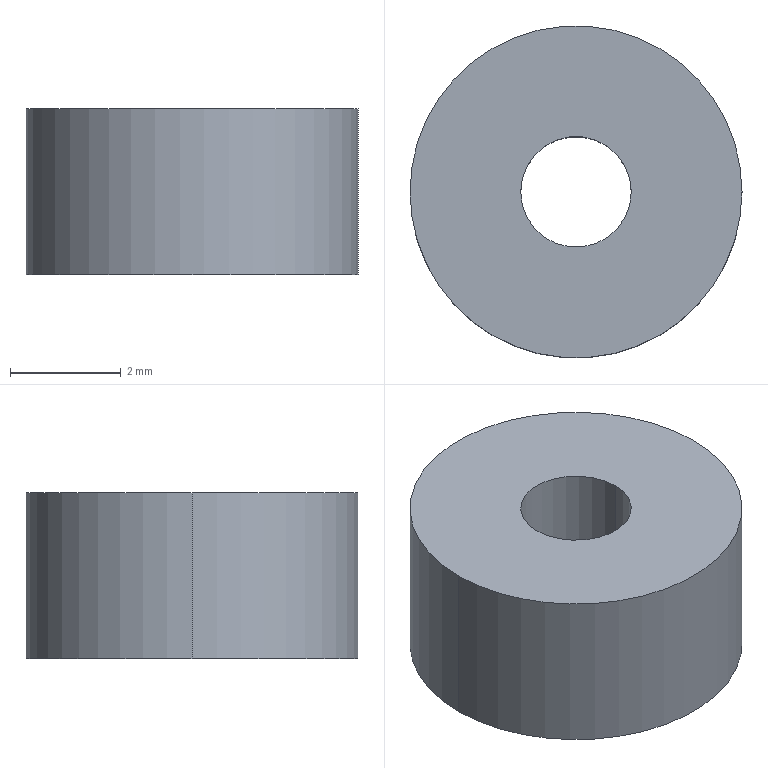Part | STEP file | 1 solid | 6 faces | box 6 x 6 x 3 mm | volume 75.398 mm3 | cylinder 4 | plane 2 | commonest cylinder face diameters 2 x2 6 x2
STEP:
#1=CARTESIAN_POINT('',(0.,0.,0.));
#2=DIRECTION('',(0.,0.,1.));
#3=DIRECTION('',(1.,0.,0.));
#4=AXIS2_PLACEMENT_3D('',#1,#2,#3);
#5=CARTESIAN_POINT('',(1.,0.,0.));
#6=VERTEX_POINT('',#5);
#7=CARTESIAN_POINT('',(-1.,0.,0.));
#8=VERTEX_POINT('',#7);
#9=CARTESIAN_POINT('',(0.,0.,0.));
#10=DIRECTION('',(0.,0.,1.));
#11=DIRECTION('',(1.,0.,0.));
#12=AXIS2_PLACEMENT_3D('',#9,#10,#11);
#13=CIRCLE('',#12,1.);
#14=CARTESIAN_POINT('',(0.,0.,3.));
#15=DIRECTION('',(0.,0.,-1.));
#16=DIRECTION('',(-1.,0.,0.));
#17=AXIS2_PLACEMENT_3D('',#14,#15,#16);
#18=CYLINDRICAL_SURFACE('',#17,1.);
#19=CARTESIAN_POINT('',(3.142,3.));
#20=DIRECTION('',(-1.,0.));
#21=VECTOR('',#20,1.);
#22=LINE('',#19,#21);
#23=(GEOMETRIC_REPRESENTATION_CONTEXT(2)PARAMETRIC_REPRESENTATION_CONTEXT()REPRESENTATION_CONTEXT('',''));
#24=DEFINITIONAL_REPRESENTATION('',(#22),#23);
#25=PCURVE('',#18,#24);
#26=CARTESIAN_POINT('',(0.,0.,0.));
#27=DIRECTION('',(0.,0.,1.));
#28=DIRECTION('',(1.,0.,0.));
#29=AXIS2_PLACEMENT_3D('',#26,#27,#28);
#30=PLANE('',#29);
#31=CARTESIAN_POINT('',(0.,0.));
#32=DIRECTION('',(1.,0.));
#33=AXIS2_PLACEMENT_2D('',#31,#32);
#34=CIRCLE('',#33,1.);
#35=(GEOMETRIC_REPRESENTATION_CONTEXT(2)PARAMETRIC_REPRESENTATION_CONTEXT()REPRESENTATION_CONTEXT('',''));
#36=DEFINITIONAL_REPRESENTATION('',(#34),#35);
#37=PCURVE('',#30,#36);
#38=SURFACE_CURVE('',#13,(#25,#37),.PCURVE_S1.);
#39=EDGE_CURVE('',#6,#8,#38,.T.);
#40=ORIENTED_EDGE('',*,*,#39,.T.);
#41=CARTESIAN_POINT('',(-1.,0.,3.));
#42=VERTEX_POINT('',#41);
#43=CARTESIAN_POINT('',(-1.,0.,3.));
#44=DIRECTION('',(0.,0.,-1.));
#45=VECTOR('',#44,1.);
#46=LINE('',#43,#45);
#47=CARTESIAN_POINT('',(0.,0.));
#48=DIRECTION('',(0.,1.));
#49=VECTOR('',#48,1.);
#50=LINE('',#47,#49);
#51=(GEOMETRIC_REPRESENTATION_CONTEXT(2)PARAMETRIC_REPRESENTATION_CONTEXT()REPRESENTATION_CONTEXT('',''));
#52=DEFINITIONAL_REPRESENTATION('',(#50),#51);
#53=PCURVE('',#18,#52);
#54=CARTESIAN_POINT('',(0.,0.,3.));
#55=DIRECTION('',(0.,0.,-1.));
#56=DIRECTION('',(-1.,0.,0.));
#57=AXIS2_PLACEMENT_3D('',#54,#55,#56);
#58=CYLINDRICAL_SURFACE('',#57,1.);
#59=CARTESIAN_POINT('',(6.283,0.));
#60=DIRECTION('',(0.,1.));
#61=VECTOR('',#60,1.);
#62=LINE('',#59,#61);
#63=(GEOMETRIC_REPRESENTATION_CONTEXT(2)PARAMETRIC_REPRESENTATION_CONTEXT()REPRESENTATION_CONTEXT('',''));
#64=DEFINITIONAL_REPRESENTATION('',(#62),#63);
#65=PCURVE('',#58,#64);
#66=SURFACE_CURVE('',#46,(#53,#65),.PCURVE_S1.);
#67=EDGE_CURVE('',#42,#8,#66,.T.);
#68=ORIENTED_EDGE('',*,*,#67,.F.);
#69=CARTESIAN_POINT('',(1.,0.,3.));
#70=VERTEX_POINT('',#69);
#71=CARTESIAN_POINT('',(0.,0.,3.));
#72=DIRECTION('',(0.,0.,1.));
#73=DIRECTION('',(1.,0.,0.));
#74=AXIS2_PLACEMENT_3D('',#71,#72,#73);
#75=CIRCLE('',#74,1.);
#76=CARTESIAN_POINT('',(3.142,0.));
#77=DIRECTION('',(-1.,0.));
#78=VECTOR('',#77,1.);
#79=LINE('',#76,#78);
#80=(GEOMETRIC_REPRESENTATION_CONTEXT(2)PARAMETRIC_REPRESENTATION_CONTEXT()REPRESENTATION_CONTEXT('',''));
#81=DEFINITIONAL_REPRESENTATION('',(#79),#80);
#82=PCURVE('',#18,#81);
#83=CARTESIAN_POINT('',(0.,0.,3.));
#84=DIRECTION('',(0.,0.,1.));
#85=DIRECTION('',(1.,0.,0.));
#86=AXIS2_PLACEMENT_3D('',#83,#84,#85);
#87=PLANE('',#86);
#88=CARTESIAN_POINT('',(0.,0.));
#89=DIRECTION('',(1.,0.));
#90=AXIS2_PLACEMENT_2D('',#88,#89);
#91=CIRCLE('',#90,1.);
#92=(GEOMETRIC_REPRESENTATION_CONTEXT(2)PARAMETRIC_REPRESENTATION_CONTEXT()REPRESENTATION_CONTEXT('',''));
#93=DEFINITIONAL_REPRESENTATION('',(#91),#92);
#94=PCURVE('',#87,#93);
#95=SURFACE_CURVE('',#75,(#82,#94),.PCURVE_S1.);
#96=EDGE_CURVE('',#70,#42,#95,.T.);
#97=ORIENTED_EDGE('',*,*,#96,.F.);
#98=CARTESIAN_POINT('',(1.,0.,3.));
#99=DIRECTION('',(0.,0.,-1.));
#100=VECTOR('',#99,1.);
#101=LINE('',#98,#100);
#102=CARTESIAN_POINT('',(3.142,0.));
#103=DIRECTION('',(0.,1.));
#104=VECTOR('',#103,1.);
#105=LINE('',#102,#104);
#106=(GEOMETRIC_REPRESENTATION_CONTEXT(2)PARAMETRIC_REPRESENTATION_CONTEXT()REPRESENTATION_CONTEXT('',''));
#107=DEFINITIONAL_REPRESENTATION('',(#105),#106);
#108=PCURVE('',#18,#107);
#109=CARTESIAN_POINT('',(3.142,0.));
#110=DIRECTION('',(0.,1.));
#111=VECTOR('',#110,1.);
#112=LINE('',#109,#111);
#113=(GEOMETRIC_REPRESENTATION_CONTEXT(2)PARAMETRIC_REPRESENTATION_CONTEXT()REPRESENTATION_CONTEXT('',''));
#114=DEFINITIONAL_REPRESENTATION('',(#112),#113);
#115=PCURVE('',#58,#114);
#116=SURFACE_CURVE('',#101,(#108,#115),.PCURVE_S1.);
#117=EDGE_CURVE('',#70,#6,#116,.T.);
#118=ORIENTED_EDGE('',*,*,#117,.T.);
#119=EDGE_LOOP('',(#40,#68,#97,#118));
#120=FACE_BOUND('',#119,.F.);
#121=ADVANCED_FACE('',(#120),#18,.F.);
#122=CARTESIAN_POINT('',(3.,0.,3.));
#123=VERTEX_POINT('',#122);
#124=CARTESIAN_POINT('',(3.,0.,0.));
#125=VERTEX_POINT('',#124);
#126=CARTESIAN_POINT('',(3.,0.,3.));
#127=DIRECTION('',(0.,0.,-1.));
#128=VECTOR('',#127,1.);
#129=LINE('',#126,#128);
#130=CARTESIAN_POINT('',(0.,0.,3.));
#131=DIRECTION('',(0.,0.,-1.));
#132=DIRECTION('',(-1.,0.,0.));
#133=AXIS2_PLACEMENT_3D('',#130,#131,#132);
#134=CYLINDRICAL_SURFACE('',#133,3.);
#135=CARTESIAN_POINT('',(3.142,0.));
#136=DIRECTION('',(0.,1.));
#137=VECTOR('',#136,1.);
#138=LINE('',#135,#137);
#139=(GEOMETRIC_REPRESENTATION_CONTEXT(2)PARAMETRIC_REPRESENTATION_CONTEXT()REPRESENTATION_CONTEXT('',''));
#140=DEFINITIONAL_REPRESENTATION('',(#138),#139);
#141=PCURVE('',#134,#140);
#142=CARTESIAN_POINT('',(0.,0.,3.));
#143=DIRECTION('',(0.,0.,-1.));
#144=DIRECTION('',(-1.,0.,0.));
#145=AXIS2_PLACEMENT_3D('',#142,#143,#144);
#146=CYLINDRICAL_SURFACE('',#145,3.);
#147=CARTESIAN_POINT('',(3.142,0.));
#148=DIRECTION('',(0.,1.));
#149=VECTOR('',#148,1.);
#150=LINE('',#147,#149);
#151=(GEOMETRIC_REPRESENTATION_CONTEXT(2)PARAMETRIC_REPRESENTATION_CONTEXT()REPRESENTATION_CONTEXT('',''));
#152=DEFINITIONAL_REPRESENTATION('',(#150),#151);
#153=PCURVE('',#146,#152);
#154=SURFACE_CURVE('',#129,(#141,#153),.PCURVE_S1.);
#155=EDGE_CURVE('',#123,#125,#154,.T.);
#156=ORIENTED_EDGE('',*,*,#155,.F.);
#157=CARTESIAN_POINT('',(-3.,0.,3.));
#158=VERTEX_POINT('',#157);
#159=CARTESIAN_POINT('',(0.,0.,3.));
#160=DIRECTION('',(0.,0.,1.));
#161=DIRECTION('',(1.,0.,0.));
#162=AXIS2_PLACEMENT_3D('',#159,#160,#161);
#163=CIRCLE('',#162,3.);
#164=CARTESIAN_POINT('',(9.425,0.));
#165=DIRECTION('',(-1.,0.));
#166=VECTOR('',#165,1.);
#167=LINE('',#164,#166);
#168=(GEOMETRIC_REPRESENTATION_CONTEXT(2)PARAMETRIC_REPRESENTATION_CONTEXT()REPRESENTATION_CONTEXT('',''));
#169=DEFINITIONAL_REPRESENTATION('',(#167),#168);
#170=PCURVE('',#134,#169);
#171=CARTESIAN_POINT('',(0.,0.));
#172=DIRECTION('',(1.,0.));
#173=AXIS2_PLACEMENT_2D('',#171,#172);
#174=CIRCLE('',#173,3.);
#175=(GEOMETRIC_REPRESENTATION_CONTEXT(2)PARAMETRIC_REPRESENTATION_CONTEXT()REPRESENTATION_CONTEXT('',''));
#176=DEFINITIONAL_REPRESENTATION('',(#174),#175);
#177=PCURVE('',#87,#176);
#178=SURFACE_CURVE('',#163,(#170,#177),.PCURVE_S1.);
#179=EDGE_CURVE('',#158,#123,#178,.T.);
#180=ORIENTED_EDGE('',*,*,#179,.F.);
#181=CARTESIAN_POINT('',(-3.,0.,0.));
#182=VERTEX_POINT('',#181);
#183=CARTESIAN_POINT('',(-3.,0.,3.));
#184=DIRECTION('',(0.,0.,-1.));
#185=VECTOR('',#184,1.);
#186=LINE('',#183,#185);
#187=CARTESIAN_POINT('',(6.283,0.));
#188=DIRECTION('',(0.,1.));
#189=VECTOR('',#188,1.);
#190=LINE('',#187,#189);
#191=(GEOMETRIC_REPRESENTATION_CONTEXT(2)PARAMETRIC_REPRESENTATION_CONTEXT()REPRESENTATION_CONTEXT('',''));
#192=DEFINITIONAL_REPRESENTATION('',(#190),#191);
#193=PCURVE('',#134,#192);
#194=CARTESIAN_POINT('',(0.,0.));
#195=DIRECTION('',(0.,1.));
#196=VECTOR('',#195,1.);
#197=LINE('',#194,#196);
#198=(GEOMETRIC_REPRESENTATION_CONTEXT(2)PARAMETRIC_REPRESENTATION_CONTEXT()REPRESENTATION_CONTEXT('',''));
#199=DEFINITIONAL_REPRESENTATION('',(#197),#198);
#200=PCURVE('',#146,#199);
#201=SURFACE_CURVE('',#186,(#193,#200),.PCURVE_S1.);
#202=EDGE_CURVE('',#158,#182,#201,.T.);
#203=ORIENTED_EDGE('',*,*,#202,.T.);
#204=CARTESIAN_POINT('',(0.,0.,0.));
#205=DIRECTION('',(0.,0.,1.));
#206=DIRECTION('',(1.,0.,0.));
#207=AXIS2_PLACEMENT_3D('',#204,#205,#206);
#208=CIRCLE('',#207,3.);
#209=CARTESIAN_POINT('',(9.425,3.));
#210=DIRECTION('',(-1.,0.));
#211=VECTOR('',#210,1.);
#212=LINE('',#209,#211);
#213=(GEOMETRIC_REPRESENTATION_CONTEXT(2)PARAMETRIC_REPRESENTATION_CONTEXT()REPRESENTATION_CONTEXT('',''));
#214=DEFINITIONAL_REPRESENTATION('',(#212),#213);
#215=PCURVE('',#134,#214);
#216=CARTESIAN_POINT('',(0.,0.));
#217=DIRECTION('',(1.,0.));
#218=AXIS2_PLACEMENT_2D('',#216,#217);
#219=CIRCLE('',#218,3.);
#220=(GEOMETRIC_REPRESENTATION_CONTEXT(2)PARAMETRIC_REPRESENTATION_CONTEXT()REPRESENTATION_CONTEXT('',''));
#221=DEFINITIONAL_REPRESENTATION('',(#219),#220);
#222=PCURVE('',#30,#221);
#223=SURFACE_CURVE('',#208,(#215,#222),.PCURVE_S1.);
#224=EDGE_CURVE('',#182,#125,#223,.T.);
#225=ORIENTED_EDGE('',*,*,#224,.T.);
#226=EDGE_LOOP('',(#156,#180,#203,#225));
#227=FACE_BOUND('',#226,.T.);
#228=ADVANCED_FACE('',(#227),#134,.T.);
#229=CARTESIAN_POINT('',(0.,0.,0.));
#230=DIRECTION('',(0.,0.,1.));
#231=DIRECTION('',(1.,0.,0.));
#232=AXIS2_PLACEMENT_3D('',#229,#230,#231);
#233=CIRCLE('',#232,1.);
#234=CARTESIAN_POINT('',(0.,0.));
#235=DIRECTION('',(1.,0.));
#236=AXIS2_PLACEMENT_2D('',#234,#235);
#237=CIRCLE('',#236,1.);
#238=(GEOMETRIC_REPRESENTATION_CONTEXT(2)PARAMETRIC_REPRESENTATION_CONTEXT()REPRESENTATION_CONTEXT('',''));
#239=DEFINITIONAL_REPRESENTATION('',(#237),#238);
#240=PCURVE('',#30,#239);
#241=CARTESIAN_POINT('',(9.425,3.));
#242=DIRECTION('',(-1.,0.));
#243=VECTOR('',#242,1.);
#244=LINE('',#241,#243);
#245=(GEOMETRIC_REPRESENTATION_CONTEXT(2)PARAMETRIC_REPRESENTATION_CONTEXT()REPRESENTATION_CONTEXT('',''));
#246=DEFINITIONAL_REPRESENTATION('',(#244),#245);
#247=PCURVE('',#58,#246);
#248=SURFACE_CURVE('',#233,(#240,#247),.PCURVE_S1.);
#249=EDGE_CURVE('',#8,#6,#248,.T.);
#250=ORIENTED_EDGE('',*,*,#249,.T.);
#251=ORIENTED_EDGE('',*,*,#39,.T.);
#252=EDGE_LOOP('',(#250,#251));
#253=FACE_BOUND('',#252,.T.);
#254=ORIENTED_EDGE('',*,*,#224,.F.);
#255=CARTESIAN_POINT('',(0.,0.,0.));
#256=DIRECTION('',(0.,0.,1.));
#257=DIRECTION('',(1.,0.,0.));
#258=AXIS2_PLACEMENT_3D('',#255,#256,#257);
#259=CIRCLE('',#258,3.);
#260=CARTESIAN_POINT('',(0.,0.));
#261=DIRECTION('',(1.,0.));
#262=AXIS2_PLACEMENT_2D('',#260,#261);
#263=CIRCLE('',#262,3.);
#264=(GEOMETRIC_REPRESENTATION_CONTEXT(2)PARAMETRIC_REPRESENTATION_CONTEXT()REPRESENTATION_CONTEXT('',''));
#265=DEFINITIONAL_REPRESENTATION('',(#263),#264);
#266=PCURVE('',#30,#265);
#267=CARTESIAN_POINT('',(3.142,3.));
#268=DIRECTION('',(-1.,0.));
#269=VECTOR('',#268,1.);
#270=LINE('',#267,#269);
#271=(GEOMETRIC_REPRESENTATION_CONTEXT(2)PARAMETRIC_REPRESENTATION_CONTEXT()REPRESENTATION_CONTEXT('',''));
#272=DEFINITIONAL_REPRESENTATION('',(#270),#271);
#273=PCURVE('',#146,#272);
#274=SURFACE_CURVE('',#259,(#266,#273),.PCURVE_S1.);
#275=EDGE_CURVE('',#125,#182,#274,.T.);
#276=ORIENTED_EDGE('',*,*,#275,.F.);
#277=EDGE_LOOP('',(#254,#276));
#278=FACE_BOUND('',#277,.T.);
#279=ADVANCED_FACE('',(#253,#278),#30,.F.);
#280=CARTESIAN_POINT('',(0.,0.,3.));
#281=DIRECTION('',(0.,0.,1.));
#282=DIRECTION('',(1.,0.,0.));
#283=AXIS2_PLACEMENT_3D('',#280,#281,#282);
#284=CIRCLE('',#283,1.);
#285=CARTESIAN_POINT('',(0.,0.));
#286=DIRECTION('',(1.,0.));
#287=AXIS2_PLACEMENT_2D('',#285,#286);
#288=CIRCLE('',#287,1.);
#289=(GEOMETRIC_REPRESENTATION_CONTEXT(2)PARAMETRIC_REPRESENTATION_CONTEXT()REPRESENTATION_CONTEXT('',''));
#290=DEFINITIONAL_REPRESENTATION('',(#288),#289);
#291=PCURVE('',#87,#290);
#292=CARTESIAN_POINT('',(9.425,0.));
#293=DIRECTION('',(-1.,0.));
#294=VECTOR('',#293,1.);
#295=LINE('',#292,#294);
#296=(GEOMETRIC_REPRESENTATION_CONTEXT(2)PARAMETRIC_REPRESENTATION_CONTEXT()REPRESENTATION_CONTEXT('',''));
#297=DEFINITIONAL_REPRESENTATION('',(#295),#296);
#298=PCURVE('',#58,#297);
#299=SURFACE_CURVE('',#284,(#291,#298),.PCURVE_S1.);
#300=EDGE_CURVE('',#42,#70,#299,.T.);
#301=ORIENTED_EDGE('',*,*,#300,.F.);
#302=ORIENTED_EDGE('',*,*,#96,.F.);
#303=EDGE_LOOP('',(#301,#302));
#304=FACE_BOUND('',#303,.T.);
#305=ORIENTED_EDGE('',*,*,#179,.T.);
#306=CARTESIAN_POINT('',(0.,0.,3.));
#307=DIRECTION('',(0.,0.,1.));
#308=DIRECTION('',(1.,0.,0.));
#309=AXIS2_PLACEMENT_3D('',#306,#307,#308);
#310=CIRCLE('',#309,3.);
#311=CARTESIAN_POINT('',(0.,0.));
#312=DIRECTION('',(1.,0.));
#313=AXIS2_PLACEMENT_2D('',#311,#312);
#314=CIRCLE('',#313,3.);
#315=(GEOMETRIC_REPRESENTATION_CONTEXT(2)PARAMETRIC_REPRESENTATION_CONTEXT()REPRESENTATION_CONTEXT('',''));
#316=DEFINITIONAL_REPRESENTATION('',(#314),#315);
#317=PCURVE('',#87,#316);
#318=CARTESIAN_POINT('',(3.142,0.));
#319=DIRECTION('',(-1.,0.));
#320=VECTOR('',#319,1.);
#321=LINE('',#318,#320);
#322=(GEOMETRIC_REPRESENTATION_CONTEXT(2)PARAMETRIC_REPRESENTATION_CONTEXT()REPRESENTATION_CONTEXT('',''));
#323=DEFINITIONAL_REPRESENTATION('',(#321),#322);
#324=PCURVE('',#146,#323);
#325=SURFACE_CURVE('',#310,(#317,#324),.PCURVE_S1.);
#326=EDGE_CURVE('',#123,#158,#325,.T.);
#327=ORIENTED_EDGE('',*,*,#326,.T.);
#328=EDGE_LOOP('',(#305,#327));
#329=FACE_BOUND('',#328,.T.);
#330=ADVANCED_FACE('',(#304,#329),#87,.T.);
#331=ORIENTED_EDGE('',*,*,#326,.F.);
#332=ORIENTED_EDGE('',*,*,#155,.T.);
#333=ORIENTED_EDGE('',*,*,#275,.T.);
#334=ORIENTED_EDGE('',*,*,#202,.F.);
#335=EDGE_LOOP('',(#331,#332,#333,#334));
#336=FACE_BOUND('',#335,.T.);
#337=ADVANCED_FACE('',(#336),#146,.T.);
#338=ORIENTED_EDGE('',*,*,#67,.T.);
#339=ORIENTED_EDGE('',*,*,#249,.T.);
#340=ORIENTED_EDGE('',*,*,#117,.F.);
#341=ORIENTED_EDGE('',*,*,#300,.F.);
#342=EDGE_LOOP('',(#338,#339,#340,#341));
#343=FACE_BOUND('',#342,.F.);
#344=ADVANCED_FACE('',(#343),#58,.F.);
#345=CLOSED_SHELL('',(#121,#228,#279,#330,#337,#344));
#346=MANIFOLD_SOLID_BREP('',#345);
#347=(LENGTH_UNIT()NAMED_UNIT(*)SI_UNIT(.MILLI.,.METRE.));
#348=UNCERTAINTY_MEASURE_WITH_UNIT(LENGTH_MEASURE(0.0000001),#347,'','');
#349=(NAMED_UNIT(*)PLANE_ANGLE_UNIT()SI_UNIT($,.RADIAN.));
#350=(NAMED_UNIT(*)SI_UNIT($,.STERADIAN.)SOLID_ANGLE_UNIT());
#351=(GEOMETRIC_REPRESENTATION_CONTEXT(3)GLOBAL_UNCERTAINTY_ASSIGNED_CONTEXT((#348))GLOBAL_UNIT_ASSIGNED_CONTEXT((#347,#349,#350))REPRESENTATION_CONTEXT('',''));
#352=ADVANCED_BREP_SHAPE_REPRESENTATION('',(#4,#346),#351);